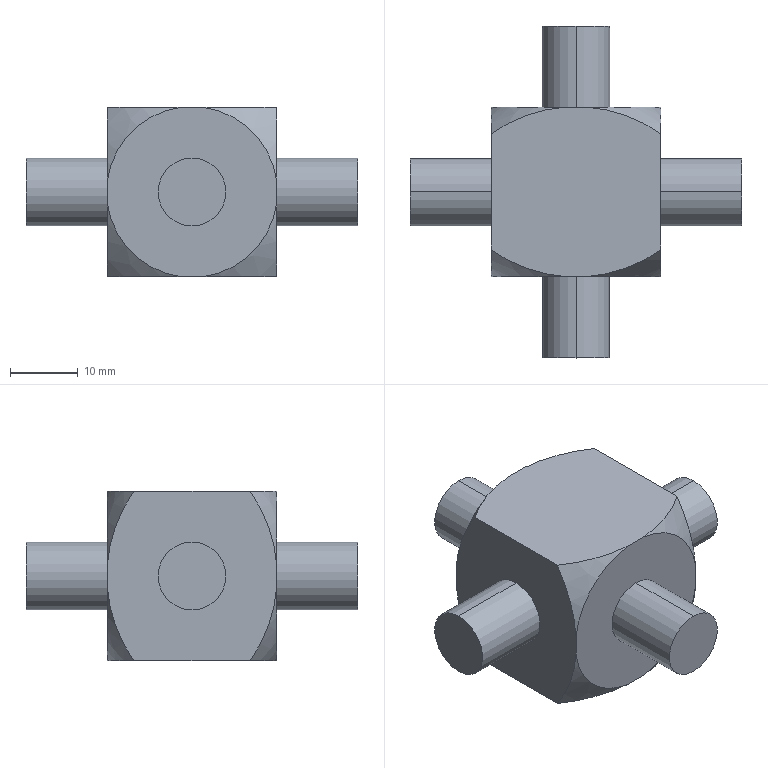Part | SolidWorks | features RefAxis 3, ICE 2, RevCut 2, 3DProfileFeature 1, Extrusion 1, LockFeature 1 | 1 solid | 26 faces | box 49 x 49 x 25 mm | volume 19131 mm3 | plane 10 | cylinder 8 | sphere 8 | commonest cylinder face diameters 10 x8
STEP:
#1=CARTESIAN_POINT('',(24.5,0.,-5.));
#2=VERTEX_POINT('',#1);
#3=CARTESIAN_POINT('',(24.5,0.,5.));
#4=VERTEX_POINT('',#3);
#5=CARTESIAN_POINT('',(24.5,0.,0.));
#6=DIRECTION('',(1.,0.,0.));
#7=DIRECTION('',(0.,0.,-1.));
#8=AXIS2_PLACEMENT_3D('',#5,#6,#7);
#9=CIRCLE('',#8,5.);
#10=EDGE_CURVE('',#2,#4,#9,.T.);
#11=ORIENTED_EDGE('',*,*,#10,.F.);
#12=CARTESIAN_POINT('',(12.5,0.,-5.));
#13=VERTEX_POINT('',#12);
#14=CARTESIAN_POINT('',(24.5,0.,-5.));
#15=DIRECTION('',(-1.,0.,0.));
#16=VECTOR('',#15,1000.);
#17=LINE('',#14,#16);
#18=EDGE_CURVE('',#2,#13,#17,.T.);
#19=ORIENTED_EDGE('',*,*,#18,.T.);
#20=CARTESIAN_POINT('',(12.5,0.,5.));
#21=VERTEX_POINT('',#20);
#22=CARTESIAN_POINT('',(12.5,0.,0.));
#23=DIRECTION('',(-1.,0.,0.));
#24=DIRECTION('',(0.,0.,-1.));
#25=AXIS2_PLACEMENT_3D('',#22,#23,#24);
#26=CIRCLE('',#25,5.);
#27=EDGE_CURVE('',#21,#13,#26,.T.);
#28=ORIENTED_EDGE('',*,*,#27,.F.);
#29=CARTESIAN_POINT('',(24.5,0.,5.));
#30=DIRECTION('',(-1.,0.,0.));
#31=VECTOR('',#30,1000.);
#32=LINE('',#29,#31);
#33=EDGE_CURVE('',#4,#21,#32,.T.);
#34=ORIENTED_EDGE('',*,*,#33,.F.);
#35=EDGE_LOOP('',(#11,#19,#28,#34));
#36=FACE_OUTER_BOUND('',#35,.T.);
#37=CARTESIAN_POINT('',(24.5,0.,0.));
#38=DIRECTION('',(-1.,0.,0.));
#39=DIRECTION('',(0.,0.,1.));
#40=AXIS2_PLACEMENT_3D('',#37,#38,#39);
#41=CYLINDRICAL_SURFACE('',#40,5.);
#42=ADVANCED_FACE('',(#36),#41,.T.);
#43=CARTESIAN_POINT('',(-12.5,0.,5.));
#44=VERTEX_POINT('',#43);
#45=CARTESIAN_POINT('',(-12.5,0.,-5.));
#46=VERTEX_POINT('',#45);
#47=CARTESIAN_POINT('',(-12.5,0.,0.));
#48=DIRECTION('',(-1.,0.,0.));
#49=DIRECTION('',(0.,0.,-1.));
#50=AXIS2_PLACEMENT_3D('',#47,#48,#49);
#51=CIRCLE('',#50,5.);
#52=EDGE_CURVE('',#44,#46,#51,.T.);
#53=ORIENTED_EDGE('',*,*,#52,.T.);
#54=CARTESIAN_POINT('',(-24.5,0.,-5.));
#55=VERTEX_POINT('',#54);
#56=CARTESIAN_POINT('',(24.5,0.,-5.));
#57=DIRECTION('',(-1.,0.,0.));
#58=VECTOR('',#57,1000.);
#59=LINE('',#56,#58);
#60=EDGE_CURVE('',#46,#55,#59,.T.);
#61=ORIENTED_EDGE('',*,*,#60,.T.);
#62=CARTESIAN_POINT('',(-24.5,0.,5.));
#63=VERTEX_POINT('',#62);
#64=CARTESIAN_POINT('',(-24.5,0.,0.));
#65=DIRECTION('',(1.,0.,0.));
#66=DIRECTION('',(0.,0.,-1.));
#67=AXIS2_PLACEMENT_3D('',#64,#65,#66);
#68=CIRCLE('',#67,5.);
#69=EDGE_CURVE('',#55,#63,#68,.T.);
#70=ORIENTED_EDGE('',*,*,#69,.T.);
#71=CARTESIAN_POINT('',(24.5,0.,5.));
#72=DIRECTION('',(-1.,0.,0.));
#73=VECTOR('',#72,1000.);
#74=LINE('',#71,#73);
#75=EDGE_CURVE('',#44,#63,#74,.T.);
#76=ORIENTED_EDGE('',*,*,#75,.F.);
#77=EDGE_LOOP('',(#53,#61,#70,#76));
#78=FACE_OUTER_BOUND('',#77,.T.);
#79=CARTESIAN_POINT('',(24.5,0.,0.));
#80=DIRECTION('',(-1.,0.,0.));
#81=DIRECTION('',(0.,0.,1.));
#82=AXIS2_PLACEMENT_3D('',#79,#80,#81);
#83=CYLINDRICAL_SURFACE('',#82,5.);
#84=ADVANCED_FACE('',(#78),#83,.T.);
#85=CARTESIAN_POINT('',(0.,24.5,5.));
#86=VERTEX_POINT('',#85);
#87=CARTESIAN_POINT('',(0.,24.5,-5.));
#88=VERTEX_POINT('',#87);
#89=CARTESIAN_POINT('',(0.,24.5,0.));
#90=DIRECTION('',(0.,1.,0.));
#91=DIRECTION('',(0.,0.,1.));
#92=AXIS2_PLACEMENT_3D('',#89,#90,#91);
#93=CIRCLE('',#92,5.);
#94=EDGE_CURVE('',#86,#88,#93,.T.);
#95=ORIENTED_EDGE('',*,*,#94,.F.);
#96=CARTESIAN_POINT('',(0.,12.5,5.));
#97=VERTEX_POINT('',#96);
#98=CARTESIAN_POINT('',(0.,24.5,5.));
#99=DIRECTION('',(0.,-1.,0.));
#100=VECTOR('',#99,1000.);
#101=LINE('',#98,#100);
#102=EDGE_CURVE('',#86,#97,#101,.T.);
#103=ORIENTED_EDGE('',*,*,#102,.T.);
#104=CARTESIAN_POINT('',(0.,12.5,-5.));
#105=VERTEX_POINT('',#104);
#106=CARTESIAN_POINT('',(0.,12.5,0.));
#107=DIRECTION('',(0.,1.,0.));
#108=DIRECTION('',(0.,0.,-1.));
#109=AXIS2_PLACEMENT_3D('',#106,#107,#108);
#110=CIRCLE('',#109,5.);
#111=EDGE_CURVE('',#97,#105,#110,.T.);
#112=ORIENTED_EDGE('',*,*,#111,.T.);
#113=CARTESIAN_POINT('',(0.,24.5,-5.));
#114=DIRECTION('',(0.,-1.,0.));
#115=VECTOR('',#114,1000.);
#116=LINE('',#113,#115);
#117=EDGE_CURVE('',#88,#105,#116,.T.);
#118=ORIENTED_EDGE('',*,*,#117,.F.);
#119=EDGE_LOOP('',(#95,#103,#112,#118));
#120=FACE_OUTER_BOUND('',#119,.T.);
#121=CARTESIAN_POINT('',(0.,24.5,0.));
#122=DIRECTION('',(0.,-1.,0.));
#123=DIRECTION('',(0.,0.,-1.));
#124=AXIS2_PLACEMENT_3D('',#121,#122,#123);
#125=CYLINDRICAL_SURFACE('',#124,5.);
#126=ADVANCED_FACE('',(#120),#125,.T.);
#127=CARTESIAN_POINT('',(0.,-12.5,-5.));
#128=VERTEX_POINT('',#127);
#129=CARTESIAN_POINT('',(0.,-12.5,5.));
#130=VERTEX_POINT('',#129);
#131=CARTESIAN_POINT('',(0.,-12.5,0.));
#132=DIRECTION('',(0.,-1.,0.));
#133=DIRECTION('',(0.,0.,1.));
#134=AXIS2_PLACEMENT_3D('',#131,#132,#133);
#135=CIRCLE('',#134,5.);
#136=EDGE_CURVE('',#128,#130,#135,.T.);
#137=ORIENTED_EDGE('',*,*,#136,.T.);
#138=CARTESIAN_POINT('',(0.,-24.5,5.));
#139=VERTEX_POINT('',#138);
#140=CARTESIAN_POINT('',(0.,24.5,5.));
#141=DIRECTION('',(0.,-1.,0.));
#142=VECTOR('',#141,1000.);
#143=LINE('',#140,#142);
#144=EDGE_CURVE('',#130,#139,#143,.T.);
#145=ORIENTED_EDGE('',*,*,#144,.T.);
#146=CARTESIAN_POINT('',(0.,-24.5,-5.));
#147=VERTEX_POINT('',#146);
#148=CARTESIAN_POINT('',(0.,-24.5,0.));
#149=DIRECTION('',(0.,1.,0.));
#150=DIRECTION('',(0.,0.,1.));
#151=AXIS2_PLACEMENT_3D('',#148,#149,#150);
#152=CIRCLE('',#151,5.);
#153=EDGE_CURVE('',#139,#147,#152,.T.);
#154=ORIENTED_EDGE('',*,*,#153,.T.);
#155=CARTESIAN_POINT('',(0.,24.5,-5.));
#156=DIRECTION('',(0.,-1.,0.));
#157=VECTOR('',#156,1000.);
#158=LINE('',#155,#157);
#159=EDGE_CURVE('',#128,#147,#158,.T.);
#160=ORIENTED_EDGE('',*,*,#159,.F.);
#161=EDGE_LOOP('',(#137,#145,#154,#160));
#162=FACE_OUTER_BOUND('',#161,.T.);
#163=CARTESIAN_POINT('',(0.,24.5,0.));
#164=DIRECTION('',(0.,-1.,0.));
#165=DIRECTION('',(0.,0.,-1.));
#166=AXIS2_PLACEMENT_3D('',#163,#164,#165);
#167=CYLINDRICAL_SURFACE('',#166,5.);
#168=ADVANCED_FACE('',(#162),#167,.T.);
#169=CARTESIAN_POINT('',(-12.5,8.587,12.5));
#170=VERTEX_POINT('',#169);
#171=CARTESIAN_POINT('',(-1.607,12.5,12.5));
#172=VERTEX_POINT('',#171);
#173=CARTESIAN_POINT('',(0.,-9.091,12.5));
#174=DIRECTION('',(0.,0.,-1.));
#175=DIRECTION('',(-1.,0.,0.));
#176=AXIS2_PLACEMENT_3D('',#173,#174,#175);
#177=CIRCLE('',#176,21.651);
#178=EDGE_CURVE('',#170,#172,#177,.T.);
#179=ORIENTED_EDGE('',*,*,#178,.F.);
#180=CARTESIAN_POINT('',(-12.5,-8.587,12.5));
#181=VERTEX_POINT('',#180);
#182=CARTESIAN_POINT('',(-12.5,12.5,12.5));
#183=DIRECTION('',(0.,-1.,0.));
#184=VECTOR('',#183,1000.);
#185=LINE('',#182,#184);
#186=EDGE_CURVE('',#170,#181,#185,.T.);
#187=ORIENTED_EDGE('',*,*,#186,.T.);
#188=CARTESIAN_POINT('',(-1.607,-12.5,12.5));
#189=VERTEX_POINT('',#188);
#190=CARTESIAN_POINT('',(0.,9.091,12.5));
#191=DIRECTION('',(0.,0.,-1.));
#192=DIRECTION('',(-1.,0.,0.));
#193=AXIS2_PLACEMENT_3D('',#190,#191,#192);
#194=CIRCLE('',#193,21.651);
#195=EDGE_CURVE('',#189,#181,#194,.T.);
#196=ORIENTED_EDGE('',*,*,#195,.F.);
#197=CARTESIAN_POINT('',(1.607,-12.5,12.5));
#198=VERTEX_POINT('',#197);
#199=CARTESIAN_POINT('',(12.5,-12.5,12.5));
#200=DIRECTION('',(-1.,0.,0.));
#201=VECTOR('',#200,1000.);
#202=LINE('',#199,#201);
#203=EDGE_CURVE('',#198,#189,#202,.T.);
#204=ORIENTED_EDGE('',*,*,#203,.F.);
#205=CARTESIAN_POINT('',(12.5,-8.587,12.5));
#206=VERTEX_POINT('',#205);
#207=CARTESIAN_POINT('',(0.,9.091,12.5));
#208=DIRECTION('',(0.,0.,-1.));
#209=DIRECTION('',(-1.,0.,0.));
#210=AXIS2_PLACEMENT_3D('',#207,#208,#209);
#211=CIRCLE('',#210,21.651);
#212=EDGE_CURVE('',#206,#198,#211,.T.);
#213=ORIENTED_EDGE('',*,*,#212,.F.);
#214=CARTESIAN_POINT('',(12.5,8.587,12.5));
#215=VERTEX_POINT('',#214);
#216=CARTESIAN_POINT('',(12.5,12.5,12.5));
#217=DIRECTION('',(0.,-1.,0.));
#218=VECTOR('',#217,1000.);
#219=LINE('',#216,#218);
#220=EDGE_CURVE('',#215,#206,#219,.T.);
#221=ORIENTED_EDGE('',*,*,#220,.F.);
#222=CARTESIAN_POINT('',(1.607,12.5,12.5));
#223=VERTEX_POINT('',#222);
#224=CARTESIAN_POINT('',(0.,-9.091,12.5));
#225=DIRECTION('',(0.,0.,-1.));
#226=DIRECTION('',(-1.,0.,0.));
#227=AXIS2_PLACEMENT_3D('',#224,#225,#226);
#228=CIRCLE('',#227,21.651);
#229=EDGE_CURVE('',#223,#215,#228,.T.);
#230=ORIENTED_EDGE('',*,*,#229,.F.);
#231=CARTESIAN_POINT('',(12.5,12.5,12.5));
#232=DIRECTION('',(-1.,0.,0.));
#233=VECTOR('',#232,1000.);
#234=LINE('',#231,#233);
#235=EDGE_CURVE('',#223,#172,#234,.T.);
#236=ORIENTED_EDGE('',*,*,#235,.T.);
#237=EDGE_LOOP('',(#179,#187,#196,#204,#213,#221,#230,#236));
#238=FACE_OUTER_BOUND('',#237,.T.);
#239=CARTESIAN_POINT('',(12.5,12.5,12.5));
#240=DIRECTION('',(0.,0.,-1.));
#241=DIRECTION('',(-1.,0.,0.));
#242=AXIS2_PLACEMENT_3D('',#239,#240,#241);
#243=PLANE('',#242);
#244=ADVANCED_FACE('',(#238),#243,.F.);
#245=CARTESIAN_POINT('',(12.5,8.587,-12.5));
#246=VERTEX_POINT('',#245);
#247=CARTESIAN_POINT('',(1.607,12.5,-12.5));
#248=VERTEX_POINT('',#247);
#249=CARTESIAN_POINT('',(0.,-9.091,-12.5));
#250=DIRECTION('',(0.,0.,1.));
#251=DIRECTION('',(1.,0.,0.));
#252=AXIS2_PLACEMENT_3D('',#249,#250,#251);
#253=CIRCLE('',#252,21.651);
#254=EDGE_CURVE('',#246,#248,#253,.T.);
#255=ORIENTED_EDGE('',*,*,#254,.F.);
#256=CARTESIAN_POINT('',(12.5,-8.587,-12.5));
#257=VERTEX_POINT('',#256);
#258=CARTESIAN_POINT('',(12.5,-12.5,-12.5));
#259=DIRECTION('',(0.,1.,0.));
#260=VECTOR('',#259,1000.);
#261=LINE('',#258,#260);
#262=EDGE_CURVE('',#257,#246,#261,.T.);
#263=ORIENTED_EDGE('',*,*,#262,.F.);
#264=CARTESIAN_POINT('',(1.607,-12.5,-12.5));
#265=VERTEX_POINT('',#264);
#266=CARTESIAN_POINT('',(0.,9.091,-12.5));
#267=DIRECTION('',(0.,0.,1.));
#268=DIRECTION('',(1.,0.,0.));
#269=AXIS2_PLACEMENT_3D('',#266,#267,#268);
#270=CIRCLE('',#269,21.651);
#271=EDGE_CURVE('',#265,#257,#270,.T.);
#272=ORIENTED_EDGE('',*,*,#271,.F.);
#273=CARTESIAN_POINT('',(-1.607,-12.5,-12.5));
#274=VERTEX_POINT('',#273);
#275=CARTESIAN_POINT('',(12.5,-12.5,-12.5));
#276=DIRECTION('',(-1.,0.,0.));
#277=VECTOR('',#276,1000.);
#278=LINE('',#275,#277);
#279=EDGE_CURVE('',#265,#274,#278,.T.);
#280=ORIENTED_EDGE('',*,*,#279,.T.);
#281=CARTESIAN_POINT('',(-12.5,-8.587,-12.5));
#282=VERTEX_POINT('',#281);
#283=CARTESIAN_POINT('',(0.,9.091,-12.5));
#284=DIRECTION('',(0.,0.,1.));
#285=DIRECTION('',(1.,0.,0.));
#286=AXIS2_PLACEMENT_3D('',#283,#284,#285);
#287=CIRCLE('',#286,21.651);
#288=EDGE_CURVE('',#282,#274,#287,.T.);
#289=ORIENTED_EDGE('',*,*,#288,.F.);
#290=CARTESIAN_POINT('',(-12.5,8.587,-12.5));
#291=VERTEX_POINT('',#290);
#292=CARTESIAN_POINT('',(-12.5,-12.5,-12.5));
#293=DIRECTION('',(0.,1.,0.));
#294=VECTOR('',#293,1000.);
#295=LINE('',#292,#294);
#296=EDGE_CURVE('',#282,#291,#295,.T.);
#297=ORIENTED_EDGE('',*,*,#296,.T.);
#298=CARTESIAN_POINT('',(-1.607,12.5,-12.5));
#299=VERTEX_POINT('',#298);
#300=CARTESIAN_POINT('',(0.,-9.091,-12.5));
#301=DIRECTION('',(0.,0.,1.));
#302=DIRECTION('',(1.,0.,0.));
#303=AXIS2_PLACEMENT_3D('',#300,#301,#302);
#304=CIRCLE('',#303,21.651);
#305=EDGE_CURVE('',#299,#291,#304,.T.);
#306=ORIENTED_EDGE('',*,*,#305,.F.);
#307=CARTESIAN_POINT('',(12.5,12.5,-12.5));
#308=DIRECTION('',(-1.,0.,0.));
#309=VECTOR('',#308,1000.);
#310=LINE('',#307,#309);
#311=EDGE_CURVE('',#248,#299,#310,.T.);
#312=ORIENTED_EDGE('',*,*,#311,.F.);
#313=EDGE_LOOP('',(#255,#263,#272,#280,#289,#297,#306,#312));
#314=FACE_OUTER_BOUND('',#313,.T.);
#315=CARTESIAN_POINT('',(12.5,-12.5,-12.5));
#316=DIRECTION('',(0.,0.,1.));
#317=DIRECTION('',(1.,0.,0.));
#318=AXIS2_PLACEMENT_3D('',#315,#316,#317);
#319=PLANE('',#318);
#320=ADVANCED_FACE('',(#314),#319,.F.);
#321=ORIENTED_EDGE('',*,*,#27,.T.);
#322=CARTESIAN_POINT('',(12.5,0.,0.));
#323=DIRECTION('',(-1.,0.,0.));
#324=DIRECTION('',(0.,0.,-1.));
#325=AXIS2_PLACEMENT_3D('',#322,#323,#324);
#326=CIRCLE('',#325,5.);
#327=EDGE_CURVE('',#13,#21,#326,.T.);
#328=ORIENTED_EDGE('',*,*,#327,.T.);
#329=EDGE_LOOP('',(#321,#328));
#330=FACE_BOUND('',#329,.T.);
#331=ORIENTED_EDGE('',*,*,#262,.T.);
#332=CARTESIAN_POINT('',(12.5,12.5,-1.607));
#333=VERTEX_POINT('',#332);
#334=CARTESIAN_POINT('',(12.5,-9.091,0.));
#335=DIRECTION('',(1.,0.,0.));
#336=DIRECTION('',(0.,0.,-1.));
#337=AXIS2_PLACEMENT_3D('',#334,#335,#336);
#338=CIRCLE('',#337,21.651);
#339=EDGE_CURVE('',#246,#333,#338,.T.);
#340=ORIENTED_EDGE('',*,*,#339,.T.);
#341=CARTESIAN_POINT('',(12.5,12.5,1.607));
#342=VERTEX_POINT('',#341);
#343=CARTESIAN_POINT('',(12.5,12.5,-12.5));
#344=DIRECTION('',(0.,0.,1.));
#345=VECTOR('',#344,1000.);
#346=LINE('',#343,#345);
#347=EDGE_CURVE('',#333,#342,#346,.T.);
#348=ORIENTED_EDGE('',*,*,#347,.T.);
#349=CARTESIAN_POINT('',(12.5,-9.091,0.));
#350=DIRECTION('',(1.,0.,0.));
#351=DIRECTION('',(0.,0.,-1.));
#352=AXIS2_PLACEMENT_3D('',#349,#350,#351);
#353=CIRCLE('',#352,21.651);
#354=EDGE_CURVE('',#342,#215,#353,.T.);
#355=ORIENTED_EDGE('',*,*,#354,.T.);
#356=ORIENTED_EDGE('',*,*,#220,.T.);
#357=CARTESIAN_POINT('',(12.5,-12.5,1.607));
#358=VERTEX_POINT('',#357);
#359=CARTESIAN_POINT('',(12.5,9.091,0.));
#360=DIRECTION('',(1.,0.,0.));
#361=DIRECTION('',(0.,0.,-1.));
#362=AXIS2_PLACEMENT_3D('',#359,#360,#361);
#363=CIRCLE('',#362,21.651);
#364=EDGE_CURVE('',#206,#358,#363,.T.);
#365=ORIENTED_EDGE('',*,*,#364,.T.);
#366=CARTESIAN_POINT('',(12.5,-12.5,-1.607));
#367=VERTEX_POINT('',#366);
#368=CARTESIAN_POINT('',(12.5,-12.5,12.5));
#369=DIRECTION('',(0.,0.,-1.));
#370=VECTOR('',#369,1000.);
#371=LINE('',#368,#370);
#372=EDGE_CURVE('',#358,#367,#371,.T.);
#373=ORIENTED_EDGE('',*,*,#372,.T.);
#374=CARTESIAN_POINT('',(12.5,9.091,0.));
#375=DIRECTION('',(1.,0.,0.));
#376=DIRECTION('',(0.,0.,-1.));
#377=AXIS2_PLACEMENT_3D('',#374,#375,#376);
#378=CIRCLE('',#377,21.651);
#379=EDGE_CURVE('',#367,#257,#378,.T.);
#380=ORIENTED_EDGE('',*,*,#379,.T.);
#381=EDGE_LOOP('',(#331,#340,#348,#355,#356,#365,#373,#380));
#382=FACE_OUTER_BOUND('',#381,.T.);
#383=CARTESIAN_POINT('',(12.5,0.,0.));
#384=DIRECTION('',(1.,0.,0.));
#385=DIRECTION('',(0.,0.,-1.));
#386=AXIS2_PLACEMENT_3D('',#383,#384,#385);
#387=PLANE('',#386);
#388=ADVANCED_FACE('',(#330,#382),#387,.T.);
#389=ORIENTED_EDGE('',*,*,#52,.F.);
#390=CARTESIAN_POINT('',(-12.5,0.,0.));
#391=DIRECTION('',(-1.,0.,0.));
#392=DIRECTION('',(0.,0.,-1.));
#393=AXIS2_PLACEMENT_3D('',#390,#391,#392);
#394=CIRCLE('',#393,5.);
#395=EDGE_CURVE('',#46,#44,#394,.T.);
#396=ORIENTED_EDGE('',*,*,#395,.F.);
#397=EDGE_LOOP('',(#389,#396));
#398=FACE_BOUND('',#397,.T.);
#399=CARTESIAN_POINT('',(-12.5,12.5,-1.607));
#400=VERTEX_POINT('',#399);
#401=CARTESIAN_POINT('',(-12.5,-9.091,0.));
#402=DIRECTION('',(1.,0.,0.));
#403=DIRECTION('',(0.,0.,-1.));
#404=AXIS2_PLACEMENT_3D('',#401,#402,#403);
#405=CIRCLE('',#404,21.651);
#406=EDGE_CURVE('',#291,#400,#405,.T.);
#407=ORIENTED_EDGE('',*,*,#406,.F.);
#408=ORIENTED_EDGE('',*,*,#296,.F.);
#409=CARTESIAN_POINT('',(-12.5,-12.5,-1.607));
#410=VERTEX_POINT('',#409);
#411=CARTESIAN_POINT('',(-12.5,9.091,0.));
#412=DIRECTION('',(1.,0.,0.));
#413=DIRECTION('',(0.,0.,-1.));
#414=AXIS2_PLACEMENT_3D('',#411,#412,#413);
#415=CIRCLE('',#414,21.651);
#416=EDGE_CURVE('',#410,#282,#415,.T.);
#417=ORIENTED_EDGE('',*,*,#416,.F.);
#418=CARTESIAN_POINT('',(-12.5,-12.5,1.607));
#419=VERTEX_POINT('',#418);
#420=CARTESIAN_POINT('',(-12.5,-12.5,12.5));
#421=DIRECTION('',(0.,0.,-1.));
#422=VECTOR('',#421,1000.);
#423=LINE('',#420,#422);
#424=EDGE_CURVE('',#419,#410,#423,.T.);
#425=ORIENTED_EDGE('',*,*,#424,.F.);
#426=CARTESIAN_POINT('',(-12.5,9.091,0.));
#427=DIRECTION('',(1.,0.,0.));
#428=DIRECTION('',(0.,0.,-1.));
#429=AXIS2_PLACEMENT_3D('',#426,#427,#428);
#430=CIRCLE('',#429,21.651);
#431=EDGE_CURVE('',#181,#419,#430,.T.);
#432=ORIENTED_EDGE('',*,*,#431,.F.);
#433=ORIENTED_EDGE('',*,*,#186,.F.);
#434=CARTESIAN_POINT('',(-12.5,12.5,1.607));
#435=VERTEX_POINT('',#434);
#436=CARTESIAN_POINT('',(-12.5,-9.091,0.));
#437=DIRECTION('',(1.,0.,0.));
#438=DIRECTION('',(0.,0.,-1.));
#439=AXIS2_PLACEMENT_3D('',#436,#437,#438);
#440=CIRCLE('',#439,21.651);
#441=EDGE_CURVE('',#435,#170,#440,.T.);
#442=ORIENTED_EDGE('',*,*,#441,.F.);
#443=CARTESIAN_POINT('',(-12.5,12.5,-12.5));
#444=DIRECTION('',(0.,0.,1.));
#445=VECTOR('',#444,1000.);
#446=LINE('',#443,#445);
#447=EDGE_CURVE('',#400,#435,#446,.T.);
#448=ORIENTED_EDGE('',*,*,#447,.F.);
#449=EDGE_LOOP('',(#407,#408,#417,#425,#432,#433,#442,#448));
#450=FACE_OUTER_BOUND('',#449,.T.);
#451=CARTESIAN_POINT('',(-12.5,0.,0.));
#452=DIRECTION('',(1.,0.,0.));
#453=DIRECTION('',(0.,0.,-1.));
#454=AXIS2_PLACEMENT_3D('',#451,#452,#453);
#455=PLANE('',#454);
#456=ADVANCED_FACE('',(#398,#450),#455,.F.);
#457=CARTESIAN_POINT('',(0.,12.5,0.));
#458=DIRECTION('',(0.,1.,0.));
#459=DIRECTION('',(0.,0.,-1.));
#460=AXIS2_PLACEMENT_3D('',#457,#458,#459);
#461=CIRCLE('',#460,5.);
#462=EDGE_CURVE('',#105,#97,#461,.T.);
#463=ORIENTED_EDGE('',*,*,#462,.F.);
#464=ORIENTED_EDGE('',*,*,#111,.F.);
#465=EDGE_LOOP('',(#463,#464));
#466=FACE_BOUND('',#465,.T.);
#467=CARTESIAN_POINT('',(0.,12.5,0.));
#468=DIRECTION('',(0.,-1.,0.));
#469=DIRECTION('',(0.,0.,-1.));
#470=AXIS2_PLACEMENT_3D('',#467,#468,#469);
#471=CIRCLE('',#470,12.603);
#472=EDGE_CURVE('',#248,#333,#471,.T.);
#473=ORIENTED_EDGE('',*,*,#472,.F.);
#474=ORIENTED_EDGE('',*,*,#311,.T.);
#475=CARTESIAN_POINT('',(0.,12.5,0.));
#476=DIRECTION('',(0.,-1.,0.));
#477=DIRECTION('',(0.,0.,-1.));
#478=AXIS2_PLACEMENT_3D('',#475,#476,#477);
#479=CIRCLE('',#478,12.603);
#480=EDGE_CURVE('',#400,#299,#479,.T.);
#481=ORIENTED_EDGE('',*,*,#480,.F.);
#482=ORIENTED_EDGE('',*,*,#447,.T.);
#483=CARTESIAN_POINT('',(0.,12.5,0.));
#484=DIRECTION('',(0.,-1.,0.));
#485=DIRECTION('',(0.,0.,-1.));
#486=AXIS2_PLACEMENT_3D('',#483,#484,#485);
#487=CIRCLE('',#486,12.603);
#488=EDGE_CURVE('',#172,#435,#487,.T.);
#489=ORIENTED_EDGE('',*,*,#488,.F.);
#490=ORIENTED_EDGE('',*,*,#235,.F.);
#491=CARTESIAN_POINT('',(0.,12.5,0.));
#492=DIRECTION('',(0.,-1.,0.));
#493=DIRECTION('',(0.,0.,-1.));
#494=AXIS2_PLACEMENT_3D('',#491,#492,#493);
#495=CIRCLE('',#494,12.603);
#496=EDGE_CURVE('',#342,#223,#495,.T.);
#497=ORIENTED_EDGE('',*,*,#496,.F.);
#498=ORIENTED_EDGE('',*,*,#347,.F.);
#499=EDGE_LOOP('',(#473,#474,#481,#482,#489,#490,#497,#498));
#500=FACE_OUTER_BOUND('',#499,.T.);
#501=CARTESIAN_POINT('',(12.5,12.5,-12.5));
#502=DIRECTION('',(0.,-1.,0.));
#503=DIRECTION('',(0.,0.,-1.));
#504=AXIS2_PLACEMENT_3D('',#501,#502,#503);
#505=PLANE('',#504);
#506=ADVANCED_FACE('',(#466,#500),#505,.F.);
#507=ORIENTED_EDGE('',*,*,#136,.F.);
#508=CARTESIAN_POINT('',(0.,-12.5,0.));
#509=DIRECTION('',(0.,-1.,0.));
#510=DIRECTION('',(0.,0.,1.));
#511=AXIS2_PLACEMENT_3D('',#508,#509,#510);
#512=CIRCLE('',#511,5.);
#513=EDGE_CURVE('',#130,#128,#512,.T.);
#514=ORIENTED_EDGE('',*,*,#513,.F.);
#515=EDGE_LOOP('',(#507,#514));
#516=FACE_BOUND('',#515,.T.);
#517=CARTESIAN_POINT('',(0.,-12.5,0.));
#518=DIRECTION('',(0.,1.,0.));
#519=DIRECTION('',(0.,0.,1.));
#520=AXIS2_PLACEMENT_3D('',#517,#518,#519);
#521=CIRCLE('',#520,12.603);
#522=EDGE_CURVE('',#198,#358,#521,.T.);
#523=ORIENTED_EDGE('',*,*,#522,.F.);
#524=ORIENTED_EDGE('',*,*,#203,.T.);
#525=CARTESIAN_POINT('',(0.,-12.5,0.));
#526=DIRECTION('',(0.,1.,0.));
#527=DIRECTION('',(0.,0.,1.));
#528=AXIS2_PLACEMENT_3D('',#525,#526,#527);
#529=CIRCLE('',#528,12.603);
#530=EDGE_CURVE('',#419,#189,#529,.T.);
#531=ORIENTED_EDGE('',*,*,#530,.F.);
#532=ORIENTED_EDGE('',*,*,#424,.T.);
#533=CARTESIAN_POINT('',(0.,-12.5,0.));
#534=DIRECTION('',(0.,1.,0.));
#535=DIRECTION('',(0.,0.,1.));
#536=AXIS2_PLACEMENT_3D('',#533,#534,#535);
#537=CIRCLE('',#536,12.603);
#538=EDGE_CURVE('',#274,#410,#537,.T.);
#539=ORIENTED_EDGE('',*,*,#538,.F.);
#540=ORIENTED_EDGE('',*,*,#279,.F.);
#541=CARTESIAN_POINT('',(0.,-12.5,0.));
#542=DIRECTION('',(0.,1.,0.));
#543=DIRECTION('',(0.,0.,1.));
#544=AXIS2_PLACEMENT_3D('',#541,#542,#543);
#545=CIRCLE('',#544,12.603);
#546=EDGE_CURVE('',#367,#265,#545,.T.);
#547=ORIENTED_EDGE('',*,*,#546,.F.);
#548=ORIENTED_EDGE('',*,*,#372,.F.);
#549=EDGE_LOOP('',(#523,#524,#531,#532,#539,#540,#547,#548));
#550=FACE_OUTER_BOUND('',#549,.T.);
#551=CARTESIAN_POINT('',(12.5,-12.5,12.5));
#552=DIRECTION('',(0.,1.,0.));
#553=DIRECTION('',(0.,0.,1.));
#554=AXIS2_PLACEMENT_3D('',#551,#552,#553);
#555=PLANE('',#554);
#556=ADVANCED_FACE('',(#516,#550),#555,.F.);
#557=ORIENTED_EDGE('',*,*,#538,.T.);
#558=ORIENTED_EDGE('',*,*,#416,.T.);
#559=ORIENTED_EDGE('',*,*,#288,.T.);
#560=EDGE_LOOP('',(#557,#558,#559));
#561=FACE_OUTER_BOUND('',#560,.T.);
#562=CARTESIAN_POINT('',(0.,9.091,0.));
#563=DIRECTION('',(-1.,0.,0.));
#564=DIRECTION('',(0.,0.,1.));
#565=AXIS2_PLACEMENT_3D('',#562,#563,#564);
#566=SPHERICAL_SURFACE('',#565,25.);
#567=ADVANCED_FACE('',(#561),#566,.T.);
#568=ORIENTED_EDGE('',*,*,#195,.T.);
#569=ORIENTED_EDGE('',*,*,#431,.T.);
#570=ORIENTED_EDGE('',*,*,#530,.T.);
#571=EDGE_LOOP('',(#568,#569,#570));
#572=FACE_OUTER_BOUND('',#571,.T.);
#573=CARTESIAN_POINT('',(0.,9.091,0.));
#574=DIRECTION('',(-1.,0.,0.));
#575=DIRECTION('',(0.,0.,1.));
#576=AXIS2_PLACEMENT_3D('',#573,#574,#575);
#577=SPHERICAL_SURFACE('',#576,25.);
#578=ADVANCED_FACE('',(#572),#577,.T.);
#579=ORIENTED_EDGE('',*,*,#546,.T.);
#580=ORIENTED_EDGE('',*,*,#271,.T.);
#581=ORIENTED_EDGE('',*,*,#379,.F.);
#582=EDGE_LOOP('',(#579,#580,#581));
#583=FACE_OUTER_BOUND('',#582,.T.);
#584=CARTESIAN_POINT('',(0.,9.091,0.));
#585=DIRECTION('',(-1.,0.,0.));
#586=DIRECTION('',(0.,0.,1.));
#587=AXIS2_PLACEMENT_3D('',#584,#585,#586);
#588=SPHERICAL_SURFACE('',#587,25.);
#589=ADVANCED_FACE('',(#583),#588,.T.);
#590=ORIENTED_EDGE('',*,*,#212,.T.);
#591=ORIENTED_EDGE('',*,*,#522,.T.);
#592=ORIENTED_EDGE('',*,*,#364,.F.);
#593=EDGE_LOOP('',(#590,#591,#592));
#594=FACE_OUTER_BOUND('',#593,.T.);
#595=CARTESIAN_POINT('',(0.,9.091,0.));
#596=DIRECTION('',(-1.,0.,0.));
#597=DIRECTION('',(0.,0.,1.));
#598=AXIS2_PLACEMENT_3D('',#595,#596,#597);
#599=SPHERICAL_SURFACE('',#598,25.);
#600=ADVANCED_FACE('',(#594),#599,.T.);
#601=ORIENTED_EDGE('',*,*,#305,.T.);
#602=ORIENTED_EDGE('',*,*,#406,.T.);
#603=ORIENTED_EDGE('',*,*,#480,.T.);
#604=EDGE_LOOP('',(#601,#602,#603));
#605=FACE_OUTER_BOUND('',#604,.T.);
#606=CARTESIAN_POINT('',(0.,-9.091,0.));
#607=DIRECTION('',(-1.,0.,0.));
#608=DIRECTION('',(0.,0.,-1.));
#609=AXIS2_PLACEMENT_3D('',#606,#607,#608);
#610=SPHERICAL_SURFACE('',#609,25.);
#611=ADVANCED_FACE('',(#605),#610,.T.);
#612=ORIENTED_EDGE('',*,*,#178,.T.);
#613=ORIENTED_EDGE('',*,*,#488,.T.);
#614=ORIENTED_EDGE('',*,*,#441,.T.);
#615=EDGE_LOOP('',(#612,#613,#614));
#616=FACE_OUTER_BOUND('',#615,.T.);
#617=CARTESIAN_POINT('',(0.,-9.091,0.));
#618=DIRECTION('',(-1.,0.,0.));
#619=DIRECTION('',(0.,0.,-1.));
#620=AXIS2_PLACEMENT_3D('',#617,#618,#619);
#621=SPHERICAL_SURFACE('',#620,25.);
#622=ADVANCED_FACE('',(#616),#621,.T.);
#623=ORIENTED_EDGE('',*,*,#229,.T.);
#624=ORIENTED_EDGE('',*,*,#354,.F.);
#625=ORIENTED_EDGE('',*,*,#496,.T.);
#626=EDGE_LOOP('',(#623,#624,#625));
#627=FACE_OUTER_BOUND('',#626,.T.);
#628=CARTESIAN_POINT('',(0.,-9.091,0.));
#629=DIRECTION('',(-1.,0.,0.));
#630=DIRECTION('',(0.,0.,-1.));
#631=AXIS2_PLACEMENT_3D('',#628,#629,#630);
#632=SPHERICAL_SURFACE('',#631,25.);
#633=ADVANCED_FACE('',(#627),#632,.T.);
#634=ORIENTED_EDGE('',*,*,#254,.T.);
#635=ORIENTED_EDGE('',*,*,#472,.T.);
#636=ORIENTED_EDGE('',*,*,#339,.F.);
#637=EDGE_LOOP('',(#634,#635,#636));
#638=FACE_OUTER_BOUND('',#637,.T.);
#639=CARTESIAN_POINT('',(0.,-9.091,0.));
#640=DIRECTION('',(-1.,0.,0.));
#641=DIRECTION('',(0.,0.,-1.));
#642=AXIS2_PLACEMENT_3D('',#639,#640,#641);
#643=SPHERICAL_SURFACE('',#642,25.);
#644=ADVANCED_FACE('',(#638),#643,.T.);
#645=CARTESIAN_POINT('',(0.,-24.5,0.));
#646=DIRECTION('',(0.,1.,0.));
#647=DIRECTION('',(0.,0.,1.));
#648=AXIS2_PLACEMENT_3D('',#645,#646,#647);
#649=CIRCLE('',#648,5.);
#650=EDGE_CURVE('',#147,#139,#649,.T.);
#651=ORIENTED_EDGE('',*,*,#650,.F.);
#652=ORIENTED_EDGE('',*,*,#153,.F.);
#653=EDGE_LOOP('',(#651,#652));
#654=FACE_OUTER_BOUND('',#653,.T.);
#655=CARTESIAN_POINT('',(0.,-24.5,0.));
#656=DIRECTION('',(0.,1.,0.));
#657=DIRECTION('',(0.,0.,1.));
#658=AXIS2_PLACEMENT_3D('',#655,#656,#657);
#659=PLANE('',#658);
#660=ADVANCED_FACE('',(#654),#659,.F.);
#661=ORIENTED_EDGE('',*,*,#144,.F.);
#662=ORIENTED_EDGE('',*,*,#513,.T.);
#663=ORIENTED_EDGE('',*,*,#159,.T.);
#664=ORIENTED_EDGE('',*,*,#650,.T.);
#665=EDGE_LOOP('',(#661,#662,#663,#664));
#666=FACE_OUTER_BOUND('',#665,.T.);
#667=CARTESIAN_POINT('',(0.,24.5,0.));
#668=DIRECTION('',(0.,-1.,0.));
#669=DIRECTION('',(0.,0.,-1.));
#670=AXIS2_PLACEMENT_3D('',#667,#668,#669);
#671=CYLINDRICAL_SURFACE('',#670,5.);
#672=ADVANCED_FACE('',(#666),#671,.T.);
#673=ORIENTED_EDGE('',*,*,#102,.F.);
#674=CARTESIAN_POINT('',(0.,24.5,0.));
#675=DIRECTION('',(0.,1.,0.));
#676=DIRECTION('',(0.,0.,1.));
#677=AXIS2_PLACEMENT_3D('',#674,#675,#676);
#678=CIRCLE('',#677,5.);
#679=EDGE_CURVE('',#88,#86,#678,.T.);
#680=ORIENTED_EDGE('',*,*,#679,.F.);
#681=ORIENTED_EDGE('',*,*,#117,.T.);
#682=ORIENTED_EDGE('',*,*,#462,.T.);
#683=EDGE_LOOP('',(#673,#680,#681,#682));
#684=FACE_OUTER_BOUND('',#683,.T.);
#685=CARTESIAN_POINT('',(0.,24.5,0.));
#686=DIRECTION('',(0.,-1.,0.));
#687=DIRECTION('',(0.,0.,-1.));
#688=AXIS2_PLACEMENT_3D('',#685,#686,#687);
#689=CYLINDRICAL_SURFACE('',#688,5.);
#690=ADVANCED_FACE('',(#684),#689,.T.);
#691=ORIENTED_EDGE('',*,*,#679,.T.);
#692=ORIENTED_EDGE('',*,*,#94,.T.);
#693=EDGE_LOOP('',(#691,#692));
#694=FACE_OUTER_BOUND('',#693,.T.);
#695=CARTESIAN_POINT('',(0.,24.5,0.));
#696=DIRECTION('',(0.,1.,0.));
#697=DIRECTION('',(0.,0.,1.));
#698=AXIS2_PLACEMENT_3D('',#695,#696,#697);
#699=PLANE('',#698);
#700=ADVANCED_FACE('',(#694),#699,.T.);
#701=CARTESIAN_POINT('',(-24.5,0.,0.));
#702=DIRECTION('',(1.,0.,0.));
#703=DIRECTION('',(0.,0.,-1.));
#704=AXIS2_PLACEMENT_3D('',#701,#702,#703);
#705=CIRCLE('',#704,5.);
#706=EDGE_CURVE('',#63,#55,#705,.T.);
#707=ORIENTED_EDGE('',*,*,#706,.F.);
#708=ORIENTED_EDGE('',*,*,#69,.F.);
#709=EDGE_LOOP('',(#707,#708));
#710=FACE_OUTER_BOUND('',#709,.T.);
#711=CARTESIAN_POINT('',(-24.5,0.,0.));
#712=DIRECTION('',(1.,0.,0.));
#713=DIRECTION('',(0.,0.,-1.));
#714=AXIS2_PLACEMENT_3D('',#711,#712,#713);
#715=PLANE('',#714);
#716=ADVANCED_FACE('',(#710),#715,.F.);
#717=ORIENTED_EDGE('',*,*,#60,.F.);
#718=ORIENTED_EDGE('',*,*,#395,.T.);
#719=ORIENTED_EDGE('',*,*,#75,.T.);
#720=ORIENTED_EDGE('',*,*,#706,.T.);
#721=EDGE_LOOP('',(#717,#718,#719,#720));
#722=FACE_OUTER_BOUND('',#721,.T.);
#723=CARTESIAN_POINT('',(24.5,0.,0.));
#724=DIRECTION('',(-1.,0.,0.));
#725=DIRECTION('',(0.,0.,1.));
#726=AXIS2_PLACEMENT_3D('',#723,#724,#725);
#727=CYLINDRICAL_SURFACE('',#726,5.);
#728=ADVANCED_FACE('',(#722),#727,.T.);
#729=ORIENTED_EDGE('',*,*,#18,.F.);
#730=CARTESIAN_POINT('',(24.5,0.,0.));
#731=DIRECTION('',(1.,0.,0.));
#732=DIRECTION('',(0.,0.,-1.));
#733=AXIS2_PLACEMENT_3D('',#730,#731,#732);
#734=CIRCLE('',#733,5.);
#735=EDGE_CURVE('',#4,#2,#734,.T.);
#736=ORIENTED_EDGE('',*,*,#735,.F.);
#737=ORIENTED_EDGE('',*,*,#33,.T.);
#738=ORIENTED_EDGE('',*,*,#327,.F.);
#739=EDGE_LOOP('',(#729,#736,#737,#738));
#740=FACE_OUTER_BOUND('',#739,.T.);
#741=CARTESIAN_POINT('',(24.5,0.,0.));
#742=DIRECTION('',(-1.,0.,0.));
#743=DIRECTION('',(0.,0.,1.));
#744=AXIS2_PLACEMENT_3D('',#741,#742,#743);
#745=CYLINDRICAL_SURFACE('',#744,5.);
#746=ADVANCED_FACE('',(#740),#745,.T.);
#747=ORIENTED_EDGE('',*,*,#735,.T.);
#748=ORIENTED_EDGE('',*,*,#10,.T.);
#749=EDGE_LOOP('',(#747,#748));
#750=FACE_OUTER_BOUND('',#749,.T.);
#751=CARTESIAN_POINT('',(24.5,0.,0.));
#752=DIRECTION('',(1.,0.,0.));
#753=DIRECTION('',(0.,0.,-1.));
#754=AXIS2_PLACEMENT_3D('',#751,#752,#753);
#755=PLANE('',#754);
#756=ADVANCED_FACE('',(#750),#755,.T.);
#757=CLOSED_SHELL('',(#42,#84,#126,#168,#244,#320,#388,#456,#506,#556,#567,#578,#589,#600,#611,#622,#633,#644,#660,#672,#690,#700,#716,#728,#746,#756));
#758=MANIFOLD_SOLID_BREP('',#757);
#759=CARTESIAN_POINT('',(0.,0.,0.));
#760=DIRECTION('',(0.,0.,1.));
#761=DIRECTION('',(1.,0.,0.));
#762=AXIS2_PLACEMENT_3D('',#759,#760,#761);
#763=(LENGTH_UNIT()NAMED_UNIT(*)SI_UNIT(.MILLI.,.METRE.));
#764=UNCERTAINTY_MEASURE_WITH_UNIT(LENGTH_MEASURE(0.00001),#763,'','');
#765=(NAMED_UNIT(*)PLANE_ANGLE_UNIT()SI_UNIT($,.RADIAN.));
#766=(NAMED_UNIT(*)SI_UNIT($,.STERADIAN.)SOLID_ANGLE_UNIT());
#767=(GEOMETRIC_REPRESENTATION_CONTEXT(3)GLOBAL_UNCERTAINTY_ASSIGNED_CONTEXT((#764))GLOBAL_UNIT_ASSIGNED_CONTEXT((#763,#765,#766))REPRESENTATION_CONTEXT('',''));
#768=ADVANCED_BREP_SHAPE_REPRESENTATION('',(#758,#762),#767);